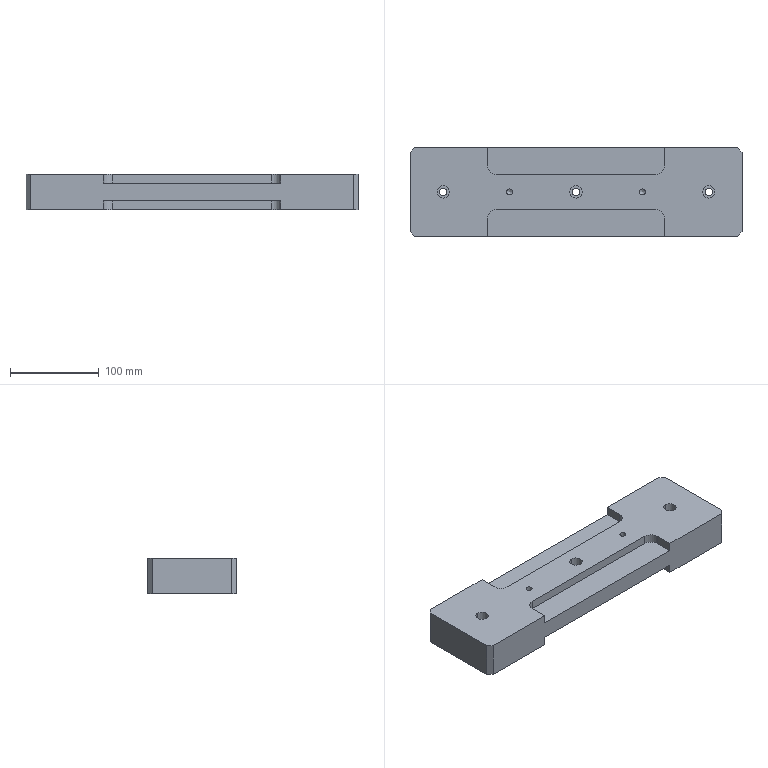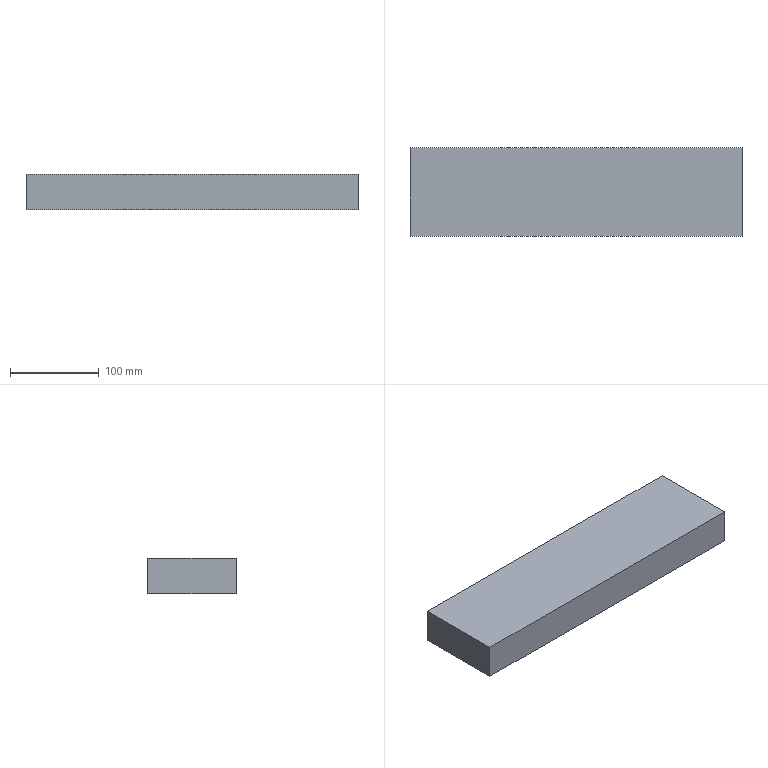CAM job | NX | 3-axis milling, drilling | part box 375 x 100 x 40 mm | stock box 375 x 100 x 40 mm
Tools:
number,name,description,diameter,corner_radius,flute_length,length,flutes
1,ZXZ,Milling Tool-5 Parameters,6.0,0.0,50.0,75.0,2
16,6.8ZT,Drilling Tool,6.8,0.0,35.0,50.0,2
17,8.5ZT,Drilling Tool,8.5,0.0,35.0,50.0,2
10,D10,Milling Tool-5 Parameters,10.0,0.0,50.0,75.0,2
21,D17R0.8,Milling Tool-5 Parameters,17.0,0.8,50.0,75.0,2
11,D10JING,Milling Tool-5 Parameters,10.0,0.0,50.0,75.0,2
22,D6A45,Milling Tool-5 Parameters,6.0,0.0,3.0,3.0,2
Operations:
program,operation,operation_type,tool,method,geometry_group,spindle_rpm,surface_speed,feed_per_tooth,feed_cut,feed_plunge,cut_length_mm,path_length_mm,cut_time_min,machine_time_min
1虎钳,DRILLING_COPY_1_COPY_1,Operation,ZXZ,METHOD,A,5000.0,94.0,0.025,250.0,0.0,20.0,412.24,0.08,0.1192
1虎钳,DRILLING_COPY_1_COPY_1_COPY,Operation,6.8ZT,METHOD,A,2000.0,31.0,0.0375,150.0,0.0,49.586,312.202,0.3306,0.3568
1虎钳,DRILLING_COPY_1_COPY_1_COPY_COPY,Operation,8.5ZT,METHOD,A,1200.0,32.0,0.0625,150.0,0.0,141.161,648.382,0.9411,0.9918
1虎钳,FLOOR_WALL,VolumeBased25DMillingOperation,D17R0.8,METHOD,A,2000.0,106.0,0.5,2000.0,1000.0,46360.028,47726.589,23.595,23.732
1虎钳,HOLE_MILLING,CylinderMilling,D10,METHOD,A,3000.0,94.0,0.2417,1450.0,100.0,3921.197,4459.697,2.704,2.758
1虎钳,ZLEVEL_PROFILE,ZLevelMilling,D10,METHOD,A,3000.0,94.0,0.3333,2000.0,100.0,16866.594,18017.943,8.433,8.548
1虎钳,FLOOR_WALL_1_1_COPY,VolumeBased25DMillingOperation,D10JING,METHOD,A,7000.0,219.0,0.0714,1000.0,100.0,3201.961,4000.874,3.202,3.282
1虎钳,ZLEVEL_PROFILE_1_COPY_1_COPY_COPY,ZLevelMilling,D6A45,METHOD,A,7500.0,141.0,0.0667,1000.0,100.0,1224.374,2518.802,1.224,1.354
1虎钳,ZLEVEL_PROFILE_1_COPY_1_COPY_COPY_COPY,ZLevelMilling,D6A45,METHOD,A,7500.0,141.0,0.0667,1000.0,100.0,397.87,662.187,0.3979,0.4243
2,FLOOR_WALL_COPY,VolumeBased25DMillingOperation,D17R0.8,METHOD,B,2000.0,106.0,0.5,2000.0,1000.0,46360.028,47726.589,23.595,23.732
2,FLOOR_WALL_1_1_COPY_COPY,VolumeBased25DMillingOperation,D10JING,METHOD,B,7000.0,219.0,0.0714,1000.0,100.0,3201.961,4000.874,3.202,3.282
2,ZLEVEL_PROFILE_1_COPY_1_COPY_COPY_COPY_1,ZLevelMilling,D6A45,METHOD,B,7500.0,141.0,0.0667,1000.0,100.0,1133.743,2070.974,1.134,1.228
2,ZLEVEL_PROFILE_1_COPY_1_COPY_COPY_COPY_COPY,ZLevelMilling,D6A45,METHOD,B,7500.0,141.0,0.0667,1000.0,100.0,397.869,662.186,0.3979,0.4243